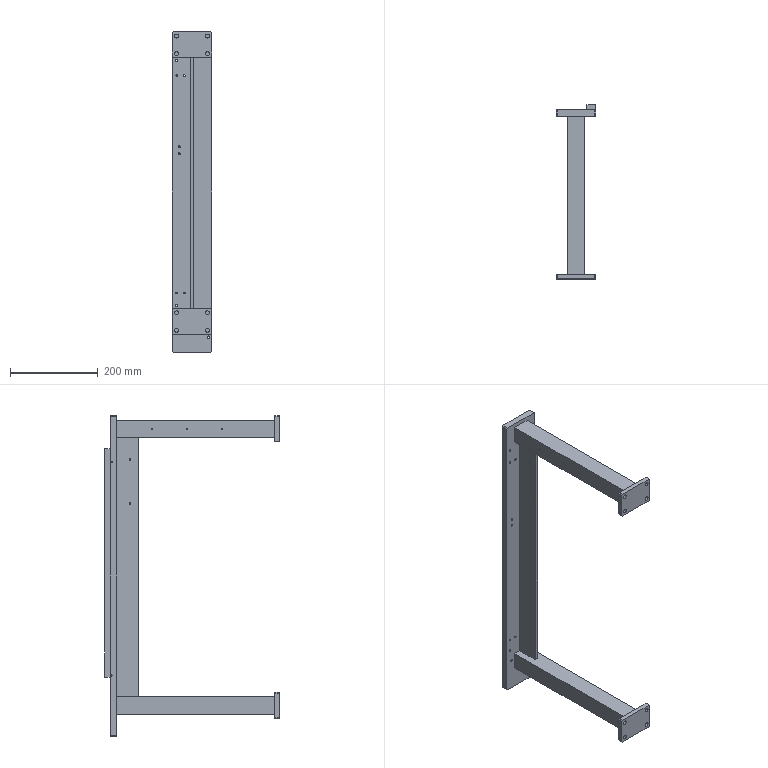Part | STEP file | 227H056235 BKT L_Default | 7 solids | 168 faces | box 90 x 397 x 730 mm | volume 1763057 mm3 | cylinder 78 | plane 62 | cone 28 | commonest cylinder face diameters 4.2 x30 3.3 x18 9 x16 5 x12 6.5 x2